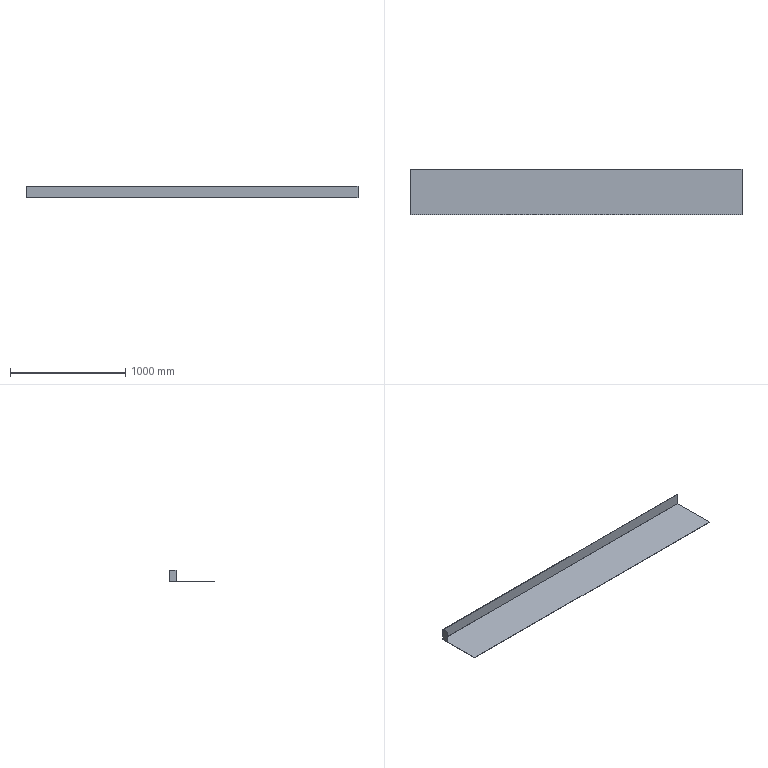Part | STEP file | PN_0036 third-floor site mounting plate 2_Default<As Machined> | 2 solids | 14 faces | box 2885 x 394 x 103 mm | volume 4292084 mm3 | plane 14
STEP:
#1=CARTESIAN_POINT('',(0.,0.,0.));
#2=DIRECTION('',(0.,0.,1.));
#3=DIRECTION('',(1.,0.,0.));
#4=AXIS2_PLACEMENT_3D('',#1,#2,#3);
#5=CARTESIAN_POINT('',(1442.5,-197.,0.));
#6=VERTEX_POINT('',#5);
#7=CARTESIAN_POINT('',(1442.5,197.,0.));
#8=VERTEX_POINT('',#7);
#9=CARTESIAN_POINT('',(1442.5,197.,0.));
#10=DIRECTION('',(0.,1.,0.));
#11=VECTOR('',#10,1.);
#12=LINE('',#9,#11);
#13=CARTESIAN_POINT('',(1442.5,197.,-3.));
#14=DIRECTION('',(1.,0.,0.));
#15=DIRECTION('',(0.,0.,-1.));
#16=AXIS2_PLACEMENT_3D('',#13,#14,#15);
#17=PLANE('',#16);
#18=CARTESIAN_POINT('',(-3.,0.));
#19=DIRECTION('',(0.,1.));
#20=VECTOR('',#19,1.);
#21=LINE('',#18,#20);
#22=(GEOMETRIC_REPRESENTATION_CONTEXT(2)PARAMETRIC_REPRESENTATION_CONTEXT()REPRESENTATION_CONTEXT('',''));
#23=DEFINITIONAL_REPRESENTATION('',(#21),#22);
#24=PCURVE('',#17,#23);
#25=CARTESIAN_POINT('',(0.,0.,0.));
#26=DIRECTION('',(0.,0.,1.));
#27=DIRECTION('',(1.,0.,0.));
#28=AXIS2_PLACEMENT_3D('',#25,#26,#27);
#29=PLANE('',#28);
#30=CARTESIAN_POINT('',(1442.5,197.));
#31=DIRECTION('',(0.,1.));
#32=VECTOR('',#31,1.);
#33=LINE('',#30,#32);
#34=(GEOMETRIC_REPRESENTATION_CONTEXT(2)PARAMETRIC_REPRESENTATION_CONTEXT()REPRESENTATION_CONTEXT('',''));
#35=DEFINITIONAL_REPRESENTATION('',(#33),#34);
#36=PCURVE('',#29,#35);
#37=SURFACE_CURVE('',#12,(#24,#36),.PCURVE_S1.);
#38=EDGE_CURVE('',#6,#8,#37,.T.);
#39=ORIENTED_EDGE('',*,*,#38,.F.);
#40=CARTESIAN_POINT('',(1442.5,-197.,-3.));
#41=VERTEX_POINT('',#40);
#42=CARTESIAN_POINT('',(1442.5,-197.,-3.));
#43=DIRECTION('',(0.,0.,1.));
#44=VECTOR('',#43,1.);
#45=LINE('',#42,#44);
#46=CARTESIAN_POINT('',(0.,-394.));
#47=DIRECTION('',(-1.,0.));
#48=VECTOR('',#47,1.);
#49=LINE('',#46,#48);
#50=(GEOMETRIC_REPRESENTATION_CONTEXT(2)PARAMETRIC_REPRESENTATION_CONTEXT()REPRESENTATION_CONTEXT('',''));
#51=DEFINITIONAL_REPRESENTATION('',(#49),#50);
#52=PCURVE('',#17,#51);
#53=CARTESIAN_POINT('',(-1442.5,-197.,-3.));
#54=DIRECTION('',(0.,-1.,0.));
#55=DIRECTION('',(0.,0.,-1.));
#56=AXIS2_PLACEMENT_3D('',#53,#54,#55);
#57=PLANE('',#56);
#58=CARTESIAN_POINT('',(0.,2885.));
#59=DIRECTION('',(-1.,0.));
#60=VECTOR('',#59,1.);
#61=LINE('',#58,#60);
#62=(GEOMETRIC_REPRESENTATION_CONTEXT(2)PARAMETRIC_REPRESENTATION_CONTEXT()REPRESENTATION_CONTEXT('',''));
#63=DEFINITIONAL_REPRESENTATION('',(#61),#62);
#64=PCURVE('',#57,#63);
#65=SURFACE_CURVE('',#45,(#52,#64),.PCURVE_S1.);
#66=EDGE_CURVE('',#41,#6,#65,.T.);
#67=ORIENTED_EDGE('',*,*,#66,.F.);
#68=CARTESIAN_POINT('',(1442.5,197.,-3.));
#69=VERTEX_POINT('',#68);
#70=CARTESIAN_POINT('',(1442.5,197.,-3.));
#71=DIRECTION('',(0.,1.,0.));
#72=VECTOR('',#71,1.);
#73=LINE('',#70,#72);
#74=CARTESIAN_POINT('',(0.,0.));
#75=DIRECTION('',(0.,1.));
#76=VECTOR('',#75,1.);
#77=LINE('',#74,#76);
#78=(GEOMETRIC_REPRESENTATION_CONTEXT(2)PARAMETRIC_REPRESENTATION_CONTEXT()REPRESENTATION_CONTEXT('',''));
#79=DEFINITIONAL_REPRESENTATION('',(#77),#78);
#80=PCURVE('',#17,#79);
#81=CARTESIAN_POINT('',(0.,0.,-3.));
#82=DIRECTION('',(0.,0.,1.));
#83=DIRECTION('',(1.,0.,0.));
#84=AXIS2_PLACEMENT_3D('',#81,#82,#83);
#85=PLANE('',#84);
#86=CARTESIAN_POINT('',(1442.5,197.));
#87=DIRECTION('',(0.,1.));
#88=VECTOR('',#87,1.);
#89=LINE('',#86,#88);
#90=(GEOMETRIC_REPRESENTATION_CONTEXT(2)PARAMETRIC_REPRESENTATION_CONTEXT()REPRESENTATION_CONTEXT('',''));
#91=DEFINITIONAL_REPRESENTATION('',(#89),#90);
#92=PCURVE('',#85,#91);
#93=SURFACE_CURVE('',#73,(#80,#92),.PCURVE_S1.);
#94=EDGE_CURVE('',#41,#69,#93,.T.);
#95=ORIENTED_EDGE('',*,*,#94,.T.);
#96=CARTESIAN_POINT('',(1442.5,197.,-3.));
#97=DIRECTION('',(0.,0.,1.));
#98=VECTOR('',#97,1.);
#99=LINE('',#96,#98);
#100=CARTESIAN_POINT('',(0.,0.));
#101=DIRECTION('',(-1.,0.));
#102=VECTOR('',#101,1.);
#103=LINE('',#100,#102);
#104=(GEOMETRIC_REPRESENTATION_CONTEXT(2)PARAMETRIC_REPRESENTATION_CONTEXT()REPRESENTATION_CONTEXT('',''));
#105=DEFINITIONAL_REPRESENTATION('',(#103),#104);
#106=PCURVE('',#17,#105);
#107=CARTESIAN_POINT('',(-1442.5,197.,-3.));
#108=DIRECTION('',(0.,1.,0.));
#109=DIRECTION('',(0.,0.,1.));
#110=AXIS2_PLACEMENT_3D('',#107,#108,#109);
#111=PLANE('',#110);
#112=CARTESIAN_POINT('',(0.,2885.));
#113=DIRECTION('',(1.,0.));
#114=VECTOR('',#113,1.);
#115=LINE('',#112,#114);
#116=(GEOMETRIC_REPRESENTATION_CONTEXT(2)PARAMETRIC_REPRESENTATION_CONTEXT()REPRESENTATION_CONTEXT('',''));
#117=DEFINITIONAL_REPRESENTATION('',(#115),#116);
#118=PCURVE('',#111,#117);
#119=SURFACE_CURVE('',#99,(#106,#118),.PCURVE_S1.);
#120=EDGE_CURVE('',#69,#8,#119,.T.);
#121=ORIENTED_EDGE('',*,*,#120,.T.);
#122=EDGE_LOOP('',(#39,#67,#95,#121));
#123=FACE_BOUND('',#122,.T.);
#124=ADVANCED_FACE('',(#123),#17,.T.);
#125=CARTESIAN_POINT('',(-1442.5,-197.,0.));
#126=VERTEX_POINT('',#125);
#127=CARTESIAN_POINT('',(-1442.5,-197.,0.));
#128=DIRECTION('',(1.,0.,0.));
#129=VECTOR('',#128,1.);
#130=LINE('',#127,#129);
#131=CARTESIAN_POINT('',(-3.,0.));
#132=DIRECTION('',(0.,1.));
#133=VECTOR('',#132,1.);
#134=LINE('',#131,#133);
#135=(GEOMETRIC_REPRESENTATION_CONTEXT(2)PARAMETRIC_REPRESENTATION_CONTEXT()REPRESENTATION_CONTEXT('',''));
#136=DEFINITIONAL_REPRESENTATION('',(#134),#135);
#137=PCURVE('',#57,#136);
#138=CARTESIAN_POINT('',(-1442.5,-197.));
#139=DIRECTION('',(1.,0.));
#140=VECTOR('',#139,1.);
#141=LINE('',#138,#140);
#142=(GEOMETRIC_REPRESENTATION_CONTEXT(2)PARAMETRIC_REPRESENTATION_CONTEXT()REPRESENTATION_CONTEXT('',''));
#143=DEFINITIONAL_REPRESENTATION('',(#141),#142);
#144=PCURVE('',#29,#143);
#145=SURFACE_CURVE('',#130,(#137,#144),.PCURVE_S1.);
#146=EDGE_CURVE('',#126,#6,#145,.T.);
#147=ORIENTED_EDGE('',*,*,#146,.F.);
#148=CARTESIAN_POINT('',(-1442.5,-197.,-3.));
#149=VERTEX_POINT('',#148);
#150=CARTESIAN_POINT('',(-1442.5,-197.,-3.));
#151=DIRECTION('',(0.,0.,1.));
#152=VECTOR('',#151,1.);
#153=LINE('',#150,#152);
#154=CARTESIAN_POINT('',(0.,0.));
#155=DIRECTION('',(-1.,0.));
#156=VECTOR('',#155,1.);
#157=LINE('',#154,#156);
#158=(GEOMETRIC_REPRESENTATION_CONTEXT(2)PARAMETRIC_REPRESENTATION_CONTEXT()REPRESENTATION_CONTEXT('',''));
#159=DEFINITIONAL_REPRESENTATION('',(#157),#158);
#160=PCURVE('',#57,#159);
#161=CARTESIAN_POINT('',(-1442.5,197.,-3.));
#162=DIRECTION('',(-1.,0.,0.));
#163=DIRECTION('',(0.,0.,1.));
#164=AXIS2_PLACEMENT_3D('',#161,#162,#163);
#165=PLANE('',#164);
#166=CARTESIAN_POINT('',(0.,-394.));
#167=DIRECTION('',(1.,0.));
#168=VECTOR('',#167,1.);
#169=LINE('',#166,#168);
#170=(GEOMETRIC_REPRESENTATION_CONTEXT(2)PARAMETRIC_REPRESENTATION_CONTEXT()REPRESENTATION_CONTEXT('',''));
#171=DEFINITIONAL_REPRESENTATION('',(#169),#170);
#172=PCURVE('',#165,#171);
#173=SURFACE_CURVE('',#153,(#160,#172),.PCURVE_S1.);
#174=EDGE_CURVE('',#149,#126,#173,.T.);
#175=ORIENTED_EDGE('',*,*,#174,.F.);
#176=CARTESIAN_POINT('',(-1442.5,-197.,-3.));
#177=DIRECTION('',(1.,0.,0.));
#178=VECTOR('',#177,1.);
#179=LINE('',#176,#178);
#180=CARTESIAN_POINT('',(0.,0.));
#181=DIRECTION('',(0.,1.));
#182=VECTOR('',#181,1.);
#183=LINE('',#180,#182);
#184=(GEOMETRIC_REPRESENTATION_CONTEXT(2)PARAMETRIC_REPRESENTATION_CONTEXT()REPRESENTATION_CONTEXT('',''));
#185=DEFINITIONAL_REPRESENTATION('',(#183),#184);
#186=PCURVE('',#57,#185);
#187=CARTESIAN_POINT('',(-1442.5,-197.));
#188=DIRECTION('',(1.,0.));
#189=VECTOR('',#188,1.);
#190=LINE('',#187,#189);
#191=(GEOMETRIC_REPRESENTATION_CONTEXT(2)PARAMETRIC_REPRESENTATION_CONTEXT()REPRESENTATION_CONTEXT('',''));
#192=DEFINITIONAL_REPRESENTATION('',(#190),#191);
#193=PCURVE('',#85,#192);
#194=SURFACE_CURVE('',#179,(#186,#193),.PCURVE_S1.);
#195=EDGE_CURVE('',#149,#41,#194,.T.);
#196=ORIENTED_EDGE('',*,*,#195,.T.);
#197=ORIENTED_EDGE('',*,*,#66,.T.);
#198=EDGE_LOOP('',(#147,#175,#196,#197));
#199=FACE_BOUND('',#198,.T.);
#200=ADVANCED_FACE('',(#199),#57,.T.);
#201=CARTESIAN_POINT('',(-1442.5,197.,0.));
#202=VERTEX_POINT('',#201);
#203=CARTESIAN_POINT('',(-1442.5,197.,0.));
#204=DIRECTION('',(0.,-1.,0.));
#205=VECTOR('',#204,1.);
#206=LINE('',#203,#205);
#207=CARTESIAN_POINT('',(3.,0.));
#208=DIRECTION('',(0.,-1.));
#209=VECTOR('',#208,1.);
#210=LINE('',#207,#209);
#211=(GEOMETRIC_REPRESENTATION_CONTEXT(2)PARAMETRIC_REPRESENTATION_CONTEXT()REPRESENTATION_CONTEXT('',''));
#212=DEFINITIONAL_REPRESENTATION('',(#210),#211);
#213=PCURVE('',#165,#212);
#214=CARTESIAN_POINT('',(-1442.5,197.));
#215=DIRECTION('',(0.,-1.));
#216=VECTOR('',#215,1.);
#217=LINE('',#214,#216);
#218=(GEOMETRIC_REPRESENTATION_CONTEXT(2)PARAMETRIC_REPRESENTATION_CONTEXT()REPRESENTATION_CONTEXT('',''));
#219=DEFINITIONAL_REPRESENTATION('',(#217),#218);
#220=PCURVE('',#29,#219);
#221=SURFACE_CURVE('',#206,(#213,#220),.PCURVE_S1.);
#222=EDGE_CURVE('',#202,#126,#221,.T.);
#223=ORIENTED_EDGE('',*,*,#222,.F.);
#224=CARTESIAN_POINT('',(-1442.5,197.,-3.));
#225=VERTEX_POINT('',#224);
#226=CARTESIAN_POINT('',(-1442.5,197.,-3.));
#227=DIRECTION('',(0.,0.,1.));
#228=VECTOR('',#227,1.);
#229=LINE('',#226,#228);
#230=CARTESIAN_POINT('',(0.,0.));
#231=DIRECTION('',(1.,0.));
#232=VECTOR('',#231,1.);
#233=LINE('',#230,#232);
#234=(GEOMETRIC_REPRESENTATION_CONTEXT(2)PARAMETRIC_REPRESENTATION_CONTEXT()REPRESENTATION_CONTEXT('',''));
#235=DEFINITIONAL_REPRESENTATION('',(#233),#234);
#236=PCURVE('',#165,#235);
#237=CARTESIAN_POINT('',(0.,0.));
#238=DIRECTION('',(1.,0.));
#239=VECTOR('',#238,1.);
#240=LINE('',#237,#239);
#241=(GEOMETRIC_REPRESENTATION_CONTEXT(2)PARAMETRIC_REPRESENTATION_CONTEXT()REPRESENTATION_CONTEXT('',''));
#242=DEFINITIONAL_REPRESENTATION('',(#240),#241);
#243=PCURVE('',#111,#242);
#244=SURFACE_CURVE('',#229,(#236,#243),.PCURVE_S1.);
#245=EDGE_CURVE('',#225,#202,#244,.T.);
#246=ORIENTED_EDGE('',*,*,#245,.F.);
#247=CARTESIAN_POINT('',(-1442.5,197.,-3.));
#248=DIRECTION('',(0.,-1.,0.));
#249=VECTOR('',#248,1.);
#250=LINE('',#247,#249);
#251=CARTESIAN_POINT('',(0.,0.));
#252=DIRECTION('',(0.,-1.));
#253=VECTOR('',#252,1.);
#254=LINE('',#251,#253);
#255=(GEOMETRIC_REPRESENTATION_CONTEXT(2)PARAMETRIC_REPRESENTATION_CONTEXT()REPRESENTATION_CONTEXT('',''));
#256=DEFINITIONAL_REPRESENTATION('',(#254),#255);
#257=PCURVE('',#165,#256);
#258=CARTESIAN_POINT('',(-1442.5,197.));
#259=DIRECTION('',(0.,-1.));
#260=VECTOR('',#259,1.);
#261=LINE('',#258,#260);
#262=(GEOMETRIC_REPRESENTATION_CONTEXT(2)PARAMETRIC_REPRESENTATION_CONTEXT()REPRESENTATION_CONTEXT('',''));
#263=DEFINITIONAL_REPRESENTATION('',(#261),#262);
#264=PCURVE('',#85,#263);
#265=SURFACE_CURVE('',#250,(#257,#264),.PCURVE_S1.);
#266=EDGE_CURVE('',#225,#149,#265,.T.);
#267=ORIENTED_EDGE('',*,*,#266,.T.);
#268=ORIENTED_EDGE('',*,*,#174,.T.);
#269=EDGE_LOOP('',(#223,#246,#267,#268));
#270=FACE_BOUND('',#269,.T.);
#271=ADVANCED_FACE('',(#270),#165,.T.);
#272=CARTESIAN_POINT('',(-1442.5,197.,0.));
#273=DIRECTION('',(-1.,0.,0.));
#274=VECTOR('',#273,1.);
#275=LINE('',#272,#274);
#276=CARTESIAN_POINT('',(3.,0.));
#277=DIRECTION('',(0.,-1.));
#278=VECTOR('',#277,1.);
#279=LINE('',#276,#278);
#280=(GEOMETRIC_REPRESENTATION_CONTEXT(2)PARAMETRIC_REPRESENTATION_CONTEXT()REPRESENTATION_CONTEXT('',''));
#281=DEFINITIONAL_REPRESENTATION('',(#279),#280);
#282=PCURVE('',#111,#281);
#283=CARTESIAN_POINT('',(-1442.5,197.));
#284=DIRECTION('',(-1.,0.));
#285=VECTOR('',#284,1.);
#286=LINE('',#283,#285);
#287=(GEOMETRIC_REPRESENTATION_CONTEXT(2)PARAMETRIC_REPRESENTATION_CONTEXT()REPRESENTATION_CONTEXT('',''));
#288=DEFINITIONAL_REPRESENTATION('',(#286),#287);
#289=PCURVE('',#29,#288);
#290=SURFACE_CURVE('',#275,(#282,#289),.PCURVE_S1.);
#291=EDGE_CURVE('',#8,#202,#290,.T.);
#292=ORIENTED_EDGE('',*,*,#291,.F.);
#293=ORIENTED_EDGE('',*,*,#120,.F.);
#294=CARTESIAN_POINT('',(-1442.5,197.,-3.));
#295=DIRECTION('',(-1.,0.,0.));
#296=VECTOR('',#295,1.);
#297=LINE('',#294,#296);
#298=CARTESIAN_POINT('',(0.,0.));
#299=DIRECTION('',(0.,-1.));
#300=VECTOR('',#299,1.);
#301=LINE('',#298,#300);
#302=(GEOMETRIC_REPRESENTATION_CONTEXT(2)PARAMETRIC_REPRESENTATION_CONTEXT()REPRESENTATION_CONTEXT('',''));
#303=DEFINITIONAL_REPRESENTATION('',(#301),#302);
#304=PCURVE('',#111,#303);
#305=CARTESIAN_POINT('',(-1442.5,197.));
#306=DIRECTION('',(-1.,0.));
#307=VECTOR('',#306,1.);
#308=LINE('',#305,#307);
#309=(GEOMETRIC_REPRESENTATION_CONTEXT(2)PARAMETRIC_REPRESENTATION_CONTEXT()REPRESENTATION_CONTEXT('',''));
#310=DEFINITIONAL_REPRESENTATION('',(#308),#309);
#311=PCURVE('',#85,#310);
#312=SURFACE_CURVE('',#297,(#304,#311),.PCURVE_S1.);
#313=EDGE_CURVE('',#69,#225,#312,.T.);
#314=ORIENTED_EDGE('',*,*,#313,.T.);
#315=ORIENTED_EDGE('',*,*,#245,.T.);
#316=EDGE_LOOP('',(#292,#293,#314,#315));
#317=FACE_BOUND('',#316,.T.);
#318=ADVANCED_FACE('',(#317),#111,.T.);
#319=ORIENTED_EDGE('',*,*,#94,.F.);
#320=ORIENTED_EDGE('',*,*,#195,.F.);
#321=ORIENTED_EDGE('',*,*,#266,.F.);
#322=ORIENTED_EDGE('',*,*,#313,.F.);
#323=EDGE_LOOP('',(#319,#320,#321,#322));
#324=FACE_BOUND('',#323,.T.);
#325=ADVANCED_FACE('',(#324),#85,.F.);
#326=ORIENTED_EDGE('',*,*,#38,.T.);
#327=ORIENTED_EDGE('',*,*,#291,.T.);
#328=ORIENTED_EDGE('',*,*,#222,.T.);
#329=ORIENTED_EDGE('',*,*,#146,.T.);
#330=EDGE_LOOP('',(#326,#327,#328,#329));
#331=FACE_BOUND('',#330,.T.);
#332=ADVANCED_FACE('',(#331),#29,.T.);
#333=CLOSED_SHELL('',(#124,#200,#271,#318,#325,#332));
#334=MANIFOLD_SOLID_BREP('',#333);
#335=CARTESIAN_POINT('',(-1442.5,197.,0.));
#336=VERTEX_POINT('',#335);
#337=CARTESIAN_POINT('',(-1442.5,138.955,0.));
#338=VERTEX_POINT('',#337);
#339=CARTESIAN_POINT('',(-1442.5,197.,0.));
#340=DIRECTION('',(0.,-1.,0.));
#341=VECTOR('',#340,1.);
#342=LINE('',#339,#341);
#343=CARTESIAN_POINT('',(-1442.5,197.,100.));
#344=DIRECTION('',(1.,0.,0.));
#345=DIRECTION('',(0.,0.,-1.));
#346=AXIS2_PLACEMENT_3D('',#343,#344,#345);
#347=PLANE('',#346);
#348=CARTESIAN_POINT('',(100.,0.));
#349=DIRECTION('',(0.,-1.));
#350=VECTOR('',#349,1.);
#351=LINE('',#348,#350);
#352=(GEOMETRIC_REPRESENTATION_CONTEXT(2)PARAMETRIC_REPRESENTATION_CONTEXT()REPRESENTATION_CONTEXT('',''));
#353=DEFINITIONAL_REPRESENTATION('',(#351),#352);
#354=PCURVE('',#347,#353);
#355=CARTESIAN_POINT('',(0.,0.,0.));
#356=DIRECTION('',(0.,0.,-1.));
#357=DIRECTION('',(-1.,0.,0.));
#358=AXIS2_PLACEMENT_3D('',#355,#356,#357);
#359=PLANE('',#358);
#360=CARTESIAN_POINT('',(1442.5,197.));
#361=DIRECTION('',(0.,-1.));
#362=VECTOR('',#361,1.);
#363=LINE('',#360,#362);
#364=(GEOMETRIC_REPRESENTATION_CONTEXT(2)PARAMETRIC_REPRESENTATION_CONTEXT()REPRESENTATION_CONTEXT('',''));
#365=DEFINITIONAL_REPRESENTATION('',(#363),#364);
#366=PCURVE('',#359,#365);
#367=SURFACE_CURVE('',#342,(#354,#366),.PCURVE_S1.);
#368=EDGE_CURVE('',#336,#338,#367,.T.);
#369=ORIENTED_EDGE('',*,*,#368,.T.);
#370=CARTESIAN_POINT('',(-1442.5,138.955,100.));
#371=VERTEX_POINT('',#370);
#372=CARTESIAN_POINT('',(-1442.5,138.955,100.));
#373=DIRECTION('',(0.,0.,-1.));
#374=VECTOR('',#373,1.);
#375=LINE('',#372,#374);
#376=CARTESIAN_POINT('',(0.,-58.045));
#377=DIRECTION('',(1.,0.));
#378=VECTOR('',#377,1.);
#379=LINE('',#376,#378);
#380=(GEOMETRIC_REPRESENTATION_CONTEXT(2)PARAMETRIC_REPRESENTATION_CONTEXT()REPRESENTATION_CONTEXT('',''));
#381=DEFINITIONAL_REPRESENTATION('',(#379),#380);
#382=PCURVE('',#347,#381);
#383=CARTESIAN_POINT('',(-1439.5,138.955,100.));
#384=DIRECTION('',(0.,-1.,0.));
#385=DIRECTION('',(0.,0.,-1.));
#386=AXIS2_PLACEMENT_3D('',#383,#384,#385);
#387=PLANE('',#386);
#388=CARTESIAN_POINT('',(0.,-3.));
#389=DIRECTION('',(1.,0.));
#390=VECTOR('',#389,1.);
#391=LINE('',#388,#390);
#392=(GEOMETRIC_REPRESENTATION_CONTEXT(2)PARAMETRIC_REPRESENTATION_CONTEXT()REPRESENTATION_CONTEXT('',''));
#393=DEFINITIONAL_REPRESENTATION('',(#391),#392);
#394=PCURVE('',#387,#393);
#395=SURFACE_CURVE('',#375,(#382,#394),.PCURVE_S1.);
#396=EDGE_CURVE('',#371,#338,#395,.T.);
#397=ORIENTED_EDGE('',*,*,#396,.F.);
#398=CARTESIAN_POINT('',(-1442.5,197.,100.));
#399=VERTEX_POINT('',#398);
#400=CARTESIAN_POINT('',(-1442.5,197.,100.));
#401=DIRECTION('',(0.,-1.,0.));
#402=VECTOR('',#401,1.);
#403=LINE('',#400,#402);
#404=CARTESIAN_POINT('',(0.,0.));
#405=DIRECTION('',(0.,-1.));
#406=VECTOR('',#405,1.);
#407=LINE('',#404,#406);
#408=(GEOMETRIC_REPRESENTATION_CONTEXT(2)PARAMETRIC_REPRESENTATION_CONTEXT()REPRESENTATION_CONTEXT('',''));
#409=DEFINITIONAL_REPRESENTATION('',(#407),#408);
#410=PCURVE('',#347,#409);
#411=CARTESIAN_POINT('',(0.,0.,100.));
#412=DIRECTION('',(0.,0.,-1.));
#413=DIRECTION('',(-1.,0.,0.));
#414=AXIS2_PLACEMENT_3D('',#411,#412,#413);
#415=PLANE('',#414);
#416=CARTESIAN_POINT('',(1442.5,197.));
#417=DIRECTION('',(0.,-1.));
#418=VECTOR('',#417,1.);
#419=LINE('',#416,#418);
#420=(GEOMETRIC_REPRESENTATION_CONTEXT(2)PARAMETRIC_REPRESENTATION_CONTEXT()REPRESENTATION_CONTEXT('',''));
#421=DEFINITIONAL_REPRESENTATION('',(#419),#420);
#422=PCURVE('',#415,#421);
#423=SURFACE_CURVE('',#403,(#410,#422),.PCURVE_S1.);
#424=EDGE_CURVE('',#399,#371,#423,.T.);
#425=ORIENTED_EDGE('',*,*,#424,.F.);
#426=CARTESIAN_POINT('',(-1442.5,197.,100.));
#427=DIRECTION('',(0.,0.,-1.));
#428=VECTOR('',#427,1.);
#429=LINE('',#426,#428);
#430=CARTESIAN_POINT('',(0.,0.));
#431=DIRECTION('',(1.,0.));
#432=VECTOR('',#431,1.);
#433=LINE('',#430,#432);
#434=(GEOMETRIC_REPRESENTATION_CONTEXT(2)PARAMETRIC_REPRESENTATION_CONTEXT()REPRESENTATION_CONTEXT('',''));
#435=DEFINITIONAL_REPRESENTATION('',(#433),#434);
#436=PCURVE('',#347,#435);
#437=CARTESIAN_POINT('',(-1442.5,197.,100.));
#438=DIRECTION('',(0.,-1.,0.));
#439=DIRECTION('',(0.,0.,-1.));
#440=AXIS2_PLACEMENT_3D('',#437,#438,#439);
#441=PLANE('',#440);
#442=CARTESIAN_POINT('',(0.,0.));
#443=DIRECTION('',(1.,0.));
#444=VECTOR('',#443,1.);
#445=LINE('',#442,#444);
#446=(GEOMETRIC_REPRESENTATION_CONTEXT(2)PARAMETRIC_REPRESENTATION_CONTEXT()REPRESENTATION_CONTEXT('',''));
#447=DEFINITIONAL_REPRESENTATION('',(#445),#446);
#448=PCURVE('',#441,#447);
#449=SURFACE_CURVE('',#429,(#436,#448),.PCURVE_S1.);
#450=EDGE_CURVE('',#399,#336,#449,.T.);
#451=ORIENTED_EDGE('',*,*,#450,.T.);
#452=EDGE_LOOP('',(#369,#397,#425,#451));
#453=FACE_BOUND('',#452,.T.);
#454=ADVANCED_FACE('',(#453),#347,.F.);
#455=CARTESIAN_POINT('',(-1439.5,138.955,0.));
#456=VERTEX_POINT('',#455);
#457=CARTESIAN_POINT('',(-1439.5,138.955,0.));
#458=DIRECTION('',(-1.,0.,0.));
#459=VECTOR('',#458,1.);
#460=LINE('',#457,#459);
#461=CARTESIAN_POINT('',(100.,0.));
#462=DIRECTION('',(0.,-1.));
#463=VECTOR('',#462,1.);
#464=LINE('',#461,#463);
#465=(GEOMETRIC_REPRESENTATION_CONTEXT(2)PARAMETRIC_REPRESENTATION_CONTEXT()REPRESENTATION_CONTEXT('',''));
#466=DEFINITIONAL_REPRESENTATION('',(#464),#465);
#467=PCURVE('',#387,#466);
#468=CARTESIAN_POINT('',(1439.5,138.955));
#469=DIRECTION('',(1.,0.));
#470=VECTOR('',#469,1.);
#471=LINE('',#468,#470);
#472=(GEOMETRIC_REPRESENTATION_CONTEXT(2)PARAMETRIC_REPRESENTATION_CONTEXT()REPRESENTATION_CONTEXT('',''));
#473=DEFINITIONAL_REPRESENTATION('',(#471),#472);
#474=PCURVE('',#359,#473);
#475=SURFACE_CURVE('',#460,(#467,#474),.PCURVE_S1.);
#476=EDGE_CURVE('',#456,#338,#475,.T.);
#477=ORIENTED_EDGE('',*,*,#476,.F.);
#478=CARTESIAN_POINT('',(-1439.5,138.955,100.));
#479=VERTEX_POINT('',#478);
#480=CARTESIAN_POINT('',(-1439.5,138.955,100.));
#481=DIRECTION('',(0.,0.,-1.));
#482=VECTOR('',#481,1.);
#483=LINE('',#480,#482);
#484=CARTESIAN_POINT('',(0.,0.));
#485=DIRECTION('',(1.,0.));
#486=VECTOR('',#485,1.);
#487=LINE('',#484,#486);
#488=(GEOMETRIC_REPRESENTATION_CONTEXT(2)PARAMETRIC_REPRESENTATION_CONTEXT()REPRESENTATION_CONTEXT('',''));
#489=DEFINITIONAL_REPRESENTATION('',(#487),#488);
#490=PCURVE('',#387,#489);
#491=CARTESIAN_POINT('',(-1439.5,197.,100.));
#492=DIRECTION('',(1.,0.,0.));
#493=DIRECTION('',(0.,0.,-1.));
#494=AXIS2_PLACEMENT_3D('',#491,#492,#493);
#495=PLANE('',#494);
#496=CARTESIAN_POINT('',(0.,-58.045));
#497=DIRECTION('',(1.,0.));
#498=VECTOR('',#497,1.);
#499=LINE('',#496,#498);
#500=(GEOMETRIC_REPRESENTATION_CONTEXT(2)PARAMETRIC_REPRESENTATION_CONTEXT()REPRESENTATION_CONTEXT('',''));
#501=DEFINITIONAL_REPRESENTATION('',(#499),#500);
#502=PCURVE('',#495,#501);
#503=SURFACE_CURVE('',#483,(#490,#502),.PCURVE_S1.);
#504=EDGE_CURVE('',#479,#456,#503,.T.);
#505=ORIENTED_EDGE('',*,*,#504,.F.);
#506=CARTESIAN_POINT('',(-1439.5,138.955,100.));
#507=DIRECTION('',(-1.,0.,0.));
#508=VECTOR('',#507,1.);
#509=LINE('',#506,#508);
#510=CARTESIAN_POINT('',(0.,0.));
#511=DIRECTION('',(0.,-1.));
#512=VECTOR('',#511,1.);
#513=LINE('',#510,#512);
#514=(GEOMETRIC_REPRESENTATION_CONTEXT(2)PARAMETRIC_REPRESENTATION_CONTEXT()REPRESENTATION_CONTEXT('',''));
#515=DEFINITIONAL_REPRESENTATION('',(#513),#514);
#516=PCURVE('',#387,#515);
#517=CARTESIAN_POINT('',(1439.5,138.955));
#518=DIRECTION('',(1.,0.));
#519=VECTOR('',#518,1.);
#520=LINE('',#517,#519);
#521=(GEOMETRIC_REPRESENTATION_CONTEXT(2)PARAMETRIC_REPRESENTATION_CONTEXT()REPRESENTATION_CONTEXT('',''));
#522=DEFINITIONAL_REPRESENTATION('',(#520),#521);
#523=PCURVE('',#415,#522);
#524=SURFACE_CURVE('',#509,(#516,#523),.PCURVE_S1.);
#525=EDGE_CURVE('',#479,#371,#524,.T.);
#526=ORIENTED_EDGE('',*,*,#525,.T.);
#527=ORIENTED_EDGE('',*,*,#396,.T.);
#528=EDGE_LOOP('',(#477,#505,#526,#527));
#529=FACE_BOUND('',#528,.T.);
#530=ADVANCED_FACE('',(#529),#387,.T.);
#531=CARTESIAN_POINT('',(-1439.5,194.,0.));
#532=VERTEX_POINT('',#531);
#533=CARTESIAN_POINT('',(-1439.5,197.,0.));
#534=DIRECTION('',(0.,-1.,0.));
#535=VECTOR('',#534,1.);
#536=LINE('',#533,#535);
#537=CARTESIAN_POINT('',(100.,0.));
#538=DIRECTION('',(0.,-1.));
#539=VECTOR('',#538,1.);
#540=LINE('',#537,#539);
#541=(GEOMETRIC_REPRESENTATION_CONTEXT(2)PARAMETRIC_REPRESENTATION_CONTEXT()REPRESENTATION_CONTEXT('',''));
#542=DEFINITIONAL_REPRESENTATION('',(#540),#541);
#543=PCURVE('',#495,#542);
#544=CARTESIAN_POINT('',(1439.5,197.));
#545=DIRECTION('',(0.,-1.));
#546=VECTOR('',#545,1.);
#547=LINE('',#544,#546);
#548=(GEOMETRIC_REPRESENTATION_CONTEXT(2)PARAMETRIC_REPRESENTATION_CONTEXT()REPRESENTATION_CONTEXT('',''));
#549=DEFINITIONAL_REPRESENTATION('',(#547),#548);
#550=PCURVE('',#359,#549);
#551=SURFACE_CURVE('',#536,(#543,#550),.PCURVE_S1.);
#552=EDGE_CURVE('',#532,#456,#551,.T.);
#553=ORIENTED_EDGE('',*,*,#552,.F.);
#554=CARTESIAN_POINT('',(-1439.5,194.,100.));
#555=VERTEX_POINT('',#554);
#556=CARTESIAN_POINT('',(-1439.5,194.,100.));
#557=DIRECTION('',(0.,0.,-1.));
#558=VECTOR('',#557,1.);
#559=LINE('',#556,#558);
#560=CARTESIAN_POINT('',(0.,-3.));
#561=DIRECTION('',(1.,0.));
#562=VECTOR('',#561,1.);
#563=LINE('',#560,#562);
#564=(GEOMETRIC_REPRESENTATION_CONTEXT(2)PARAMETRIC_REPRESENTATION_CONTEXT()REPRESENTATION_CONTEXT('',''));
#565=DEFINITIONAL_REPRESENTATION('',(#563),#564);
#566=PCURVE('',#495,#565);
#567=CARTESIAN_POINT('',(-1442.5,194.,100.));
#568=DIRECTION('',(0.,-1.,0.));
#569=DIRECTION('',(0.,0.,-1.));
#570=AXIS2_PLACEMENT_3D('',#567,#568,#569);
#571=PLANE('',#570);
#572=CARTESIAN_POINT('',(0.,3.));
#573=DIRECTION('',(1.,0.));
#574=VECTOR('',#573,1.);
#575=LINE('',#572,#574);
#576=(GEOMETRIC_REPRESENTATION_CONTEXT(2)PARAMETRIC_REPRESENTATION_CONTEXT()REPRESENTATION_CONTEXT('',''));
#577=DEFINITIONAL_REPRESENTATION('',(#575),#576);
#578=PCURVE('',#571,#577);
#579=SURFACE_CURVE('',#559,(#566,#578),.PCURVE_S1.);
#580=EDGE_CURVE('',#555,#532,#579,.T.);
#581=ORIENTED_EDGE('',*,*,#580,.F.);
#582=CARTESIAN_POINT('',(-1439.5,197.,100.));
#583=DIRECTION('',(0.,-1.,0.));
#584=VECTOR('',#583,1.);
#585=LINE('',#582,#584);
#586=CARTESIAN_POINT('',(0.,0.));
#587=DIRECTION('',(0.,-1.));
#588=VECTOR('',#587,1.);
#589=LINE('',#586,#588);
#590=(GEOMETRIC_REPRESENTATION_CONTEXT(2)PARAMETRIC_REPRESENTATION_CONTEXT()REPRESENTATION_CONTEXT('',''));
#591=DEFINITIONAL_REPRESENTATION('',(#589),#590);
#592=PCURVE('',#495,#591);
#593=CARTESIAN_POINT('',(1439.5,197.));
#594=DIRECTION('',(0.,-1.));
#595=VECTOR('',#594,1.);
#596=LINE('',#593,#595);
#597=(GEOMETRIC_REPRESENTATION_CONTEXT(2)PARAMETRIC_REPRESENTATION_CONTEXT()REPRESENTATION_CONTEXT('',''));
#598=DEFINITIONAL_REPRESENTATION('',(#596),#597);
#599=PCURVE('',#415,#598);
#600=SURFACE_CURVE('',#585,(#592,#599),.PCURVE_S1.);
#601=EDGE_CURVE('',#555,#479,#600,.T.);
#602=ORIENTED_EDGE('',*,*,#601,.T.);
#603=ORIENTED_EDGE('',*,*,#504,.T.);
#604=EDGE_LOOP('',(#553,#581,#602,#603));
#605=FACE_BOUND('',#604,.T.);
#606=ADVANCED_FACE('',(#605),#495,.T.);
#607=CARTESIAN_POINT('',(1442.5,194.,0.));
#608=VERTEX_POINT('',#607);
#609=CARTESIAN_POINT('',(-1442.5,194.,0.));
#610=DIRECTION('',(-1.,0.,0.));
#611=VECTOR('',#610,1.);
#612=LINE('',#609,#611);
#613=CARTESIAN_POINT('',(100.,0.));
#614=DIRECTION('',(0.,-1.));
#615=VECTOR('',#614,1.);
#616=LINE('',#613,#615);
#617=(GEOMETRIC_REPRESENTATION_CONTEXT(2)PARAMETRIC_REPRESENTATION_CONTEXT()REPRESENTATION_CONTEXT('',''));
#618=DEFINITIONAL_REPRESENTATION('',(#616),#617);
#619=PCURVE('',#571,#618);
#620=CARTESIAN_POINT('',(1442.5,194.));
#621=DIRECTION('',(1.,0.));
#622=VECTOR('',#621,1.);
#623=LINE('',#620,#622);
#624=(GEOMETRIC_REPRESENTATION_CONTEXT(2)PARAMETRIC_REPRESENTATION_CONTEXT()REPRESENTATION_CONTEXT('',''));
#625=DEFINITIONAL_REPRESENTATION('',(#623),#624);
#626=PCURVE('',#359,#625);
#627=SURFACE_CURVE('',#612,(#619,#626),.PCURVE_S1.);
#628=EDGE_CURVE('',#608,#532,#627,.T.);
#629=ORIENTED_EDGE('',*,*,#628,.F.);
#630=CARTESIAN_POINT('',(1442.5,194.,100.));
#631=VERTEX_POINT('',#630);
#632=CARTESIAN_POINT('',(1442.5,194.,100.));
#633=DIRECTION('',(0.,0.,-1.));
#634=VECTOR('',#633,1.);
#635=LINE('',#632,#634);
#636=CARTESIAN_POINT('',(0.,2885.));
#637=DIRECTION('',(1.,0.));
#638=VECTOR('',#637,1.);
#639=LINE('',#636,#638);
#640=(GEOMETRIC_REPRESENTATION_CONTEXT(2)PARAMETRIC_REPRESENTATION_CONTEXT()REPRESENTATION_CONTEXT('',''));
#641=DEFINITIONAL_REPRESENTATION('',(#639),#640);
#642=PCURVE('',#571,#641);
#643=CARTESIAN_POINT('',(1442.5,197.,100.));
#644=DIRECTION('',(1.,0.,0.));
#645=DIRECTION('',(0.,0.,-1.));
#646=AXIS2_PLACEMENT_3D('',#643,#644,#645);
#647=PLANE('',#646);
#648=CARTESIAN_POINT('',(0.,-3.));
#649=DIRECTION('',(1.,0.));
#650=VECTOR('',#649,1.);
#651=LINE('',#648,#650);
#652=(GEOMETRIC_REPRESENTATION_CONTEXT(2)PARAMETRIC_REPRESENTATION_CONTEXT()REPRESENTATION_CONTEXT('',''));
#653=DEFINITIONAL_REPRESENTATION('',(#651),#652);
#654=PCURVE('',#647,#653);
#655=SURFACE_CURVE('',#635,(#642,#654),.PCURVE_S1.);
#656=EDGE_CURVE('',#631,#608,#655,.T.);
#657=ORIENTED_EDGE('',*,*,#656,.F.);
#658=CARTESIAN_POINT('',(-1442.5,194.,100.));
#659=DIRECTION('',(-1.,0.,0.));
#660=VECTOR('',#659,1.);
#661=LINE('',#658,#660);
#662=CARTESIAN_POINT('',(0.,0.));
#663=DIRECTION('',(0.,-1.));
#664=VECTOR('',#663,1.);
#665=LINE('',#662,#664);
#666=(GEOMETRIC_REPRESENTATION_CONTEXT(2)PARAMETRIC_REPRESENTATION_CONTEXT()REPRESENTATION_CONTEXT('',''));
#667=DEFINITIONAL_REPRESENTATION('',(#665),#666);
#668=PCURVE('',#571,#667);
#669=CARTESIAN_POINT('',(1442.5,194.));
#670=DIRECTION('',(1.,0.));
#671=VECTOR('',#670,1.);
#672=LINE('',#669,#671);
#673=(GEOMETRIC_REPRESENTATION_CONTEXT(2)PARAMETRIC_REPRESENTATION_CONTEXT()REPRESENTATION_CONTEXT('',''));
#674=DEFINITIONAL_REPRESENTATION('',(#672),#673);
#675=PCURVE('',#415,#674);
#676=SURFACE_CURVE('',#661,(#668,#675),.PCURVE_S1.);
#677=EDGE_CURVE('',#631,#555,#676,.T.);
#678=ORIENTED_EDGE('',*,*,#677,.T.);
#679=ORIENTED_EDGE('',*,*,#580,.T.);
#680=EDGE_LOOP('',(#629,#657,#678,#679));
#681=FACE_BOUND('',#680,.T.);
#682=ADVANCED_FACE('',(#681),#571,.T.);
#683=CARTESIAN_POINT('',(1442.5,197.,0.));
#684=VERTEX_POINT('',#683);
#685=CARTESIAN_POINT('',(1442.5,197.,0.));
#686=DIRECTION('',(0.,-1.,0.));
#687=VECTOR('',#686,1.);
#688=LINE('',#685,#687);
#689=CARTESIAN_POINT('',(100.,0.));
#690=DIRECTION('',(0.,-1.));
#691=VECTOR('',#690,1.);
#692=LINE('',#689,#691);
#693=(GEOMETRIC_REPRESENTATION_CONTEXT(2)PARAMETRIC_REPRESENTATION_CONTEXT()REPRESENTATION_CONTEXT('',''));
#694=DEFINITIONAL_REPRESENTATION('',(#692),#693);
#695=PCURVE('',#647,#694);
#696=CARTESIAN_POINT('',(-1442.5,197.));
#697=DIRECTION('',(0.,-1.));
#698=VECTOR('',#697,1.);
#699=LINE('',#696,#698);
#700=(GEOMETRIC_REPRESENTATION_CONTEXT(2)PARAMETRIC_REPRESENTATION_CONTEXT()REPRESENTATION_CONTEXT('',''));
#701=DEFINITIONAL_REPRESENTATION('',(#699),#700);
#702=PCURVE('',#359,#701);
#703=SURFACE_CURVE('',#688,(#695,#702),.PCURVE_S1.);
#704=EDGE_CURVE('',#684,#608,#703,.T.);
#705=ORIENTED_EDGE('',*,*,#704,.F.);
#706=CARTESIAN_POINT('',(1442.5,197.,100.));
#707=VERTEX_POINT('',#706);
#708=CARTESIAN_POINT('',(1442.5,197.,100.));
#709=DIRECTION('',(0.,0.,-1.));
#710=VECTOR('',#709,1.);
#711=LINE('',#708,#710);
#712=CARTESIAN_POINT('',(0.,0.));
#713=DIRECTION('',(1.,0.));
#714=VECTOR('',#713,1.);
#715=LINE('',#712,#714);
#716=(GEOMETRIC_REPRESENTATION_CONTEXT(2)PARAMETRIC_REPRESENTATION_CONTEXT()REPRESENTATION_CONTEXT('',''));
#717=DEFINITIONAL_REPRESENTATION('',(#715),#716);
#718=PCURVE('',#647,#717);
#719=CARTESIAN_POINT('',(0.,2885.));
#720=DIRECTION('',(1.,0.));
#721=VECTOR('',#720,1.);
#722=LINE('',#719,#721);
#723=(GEOMETRIC_REPRESENTATION_CONTEXT(2)PARAMETRIC_REPRESENTATION_CONTEXT()REPRESENTATION_CONTEXT('',''));
#724=DEFINITIONAL_REPRESENTATION('',(#722),#723);
#725=PCURVE('',#441,#724);
#726=SURFACE_CURVE('',#711,(#718,#725),.PCURVE_S1.);
#727=EDGE_CURVE('',#707,#684,#726,.T.);
#728=ORIENTED_EDGE('',*,*,#727,.F.);
#729=CARTESIAN_POINT('',(1442.5,197.,100.));
#730=DIRECTION('',(0.,-1.,0.));
#731=VECTOR('',#730,1.);
#732=LINE('',#729,#731);
#733=CARTESIAN_POINT('',(0.,0.));
#734=DIRECTION('',(0.,-1.));
#735=VECTOR('',#734,1.);
#736=LINE('',#733,#735);
#737=(GEOMETRIC_REPRESENTATION_CONTEXT(2)PARAMETRIC_REPRESENTATION_CONTEXT()REPRESENTATION_CONTEXT('',''));
#738=DEFINITIONAL_REPRESENTATION('',(#736),#737);
#739=PCURVE('',#647,#738);
#740=CARTESIAN_POINT('',(-1442.5,197.));
#741=DIRECTION('',(0.,-1.));
#742=VECTOR('',#741,1.);
#743=LINE('',#740,#742);
#744=(GEOMETRIC_REPRESENTATION_CONTEXT(2)PARAMETRIC_REPRESENTATION_CONTEXT()REPRESENTATION_CONTEXT('',''));
#745=DEFINITIONAL_REPRESENTATION('',(#743),#744);
#746=PCURVE('',#415,#745);
#747=SURFACE_CURVE('',#732,(#739,#746),.PCURVE_S1.);
#748=EDGE_CURVE('',#707,#631,#747,.T.);
#749=ORIENTED_EDGE('',*,*,#748,.T.);
#750=ORIENTED_EDGE('',*,*,#656,.T.);
#751=EDGE_LOOP('',(#705,#728,#749,#750));
#752=FACE_BOUND('',#751,.T.);
#753=ADVANCED_FACE('',(#752),#647,.T.);
#754=CARTESIAN_POINT('',(-1442.5,197.,0.));
#755=DIRECTION('',(-1.,0.,0.));
#756=VECTOR('',#755,1.);
#757=LINE('',#754,#756);
#758=CARTESIAN_POINT('',(100.,0.));
#759=DIRECTION('',(0.,-1.));
#760=VECTOR('',#759,1.);
#761=LINE('',#758,#760);
#762=(GEOMETRIC_REPRESENTATION_CONTEXT(2)PARAMETRIC_REPRESENTATION_CONTEXT()REPRESENTATION_CONTEXT('',''));
#763=DEFINITIONAL_REPRESENTATION('',(#761),#762);
#764=PCURVE('',#441,#763);
#765=CARTESIAN_POINT('',(1442.5,197.));
#766=DIRECTION('',(1.,0.));
#767=VECTOR('',#766,1.);
#768=LINE('',#765,#767);
#769=(GEOMETRIC_REPRESENTATION_CONTEXT(2)PARAMETRIC_REPRESENTATION_CONTEXT()REPRESENTATION_CONTEXT('',''));
#770=DEFINITIONAL_REPRESENTATION('',(#768),#769);
#771=PCURVE('',#359,#770);
#772=SURFACE_CURVE('',#757,(#764,#771),.PCURVE_S1.);
#773=EDGE_CURVE('',#684,#336,#772,.T.);
#774=ORIENTED_EDGE('',*,*,#773,.T.);
#775=ORIENTED_EDGE('',*,*,#450,.F.);
#776=CARTESIAN_POINT('',(-1442.5,197.,100.));
#777=DIRECTION('',(-1.,0.,0.));
#778=VECTOR('',#777,1.);
#779=LINE('',#776,#778);
#780=CARTESIAN_POINT('',(0.,0.));
#781=DIRECTION('',(0.,-1.));
#782=VECTOR('',#781,1.);
#783=LINE('',#780,#782);
#784=(GEOMETRIC_REPRESENTATION_CONTEXT(2)PARAMETRIC_REPRESENTATION_CONTEXT()REPRESENTATION_CONTEXT('',''));
#785=DEFINITIONAL_REPRESENTATION('',(#783),#784);
#786=PCURVE('',#441,#785);
#787=CARTESIAN_POINT('',(1442.5,197.));
#788=DIRECTION('',(1.,0.));
#789=VECTOR('',#788,1.);
#790=LINE('',#787,#789);
#791=(GEOMETRIC_REPRESENTATION_CONTEXT(2)PARAMETRIC_REPRESENTATION_CONTEXT()REPRESENTATION_CONTEXT('',''));
#792=DEFINITIONAL_REPRESENTATION('',(#790),#791);
#793=PCURVE('',#415,#792);
#794=SURFACE_CURVE('',#779,(#786,#793),.PCURVE_S1.);
#795=EDGE_CURVE('',#707,#399,#794,.T.);
#796=ORIENTED_EDGE('',*,*,#795,.F.);
#797=ORIENTED_EDGE('',*,*,#727,.T.);
#798=EDGE_LOOP('',(#774,#775,#796,#797));
#799=FACE_BOUND('',#798,.T.);
#800=ADVANCED_FACE('',(#799),#441,.F.);
#801=ORIENTED_EDGE('',*,*,#424,.T.);
#802=ORIENTED_EDGE('',*,*,#525,.F.);
#803=ORIENTED_EDGE('',*,*,#601,.F.);
#804=ORIENTED_EDGE('',*,*,#677,.F.);
#805=ORIENTED_EDGE('',*,*,#748,.F.);
#806=ORIENTED_EDGE('',*,*,#795,.T.);
#807=EDGE_LOOP('',(#801,#802,#803,#804,#805,#806));
#808=FACE_BOUND('',#807,.T.);
#809=ADVANCED_FACE('',(#808),#415,.F.);
#810=ORIENTED_EDGE('',*,*,#368,.F.);
#811=ORIENTED_EDGE('',*,*,#773,.F.);
#812=ORIENTED_EDGE('',*,*,#704,.T.);
#813=ORIENTED_EDGE('',*,*,#628,.T.);
#814=ORIENTED_EDGE('',*,*,#552,.T.);
#815=ORIENTED_EDGE('',*,*,#476,.T.);
#816=EDGE_LOOP('',(#810,#811,#812,#813,#814,#815));
#817=FACE_BOUND('',#816,.T.);
#818=ADVANCED_FACE('',(#817),#359,.T.);
#819=CLOSED_SHELL('',(#454,#530,#606,#682,#753,#800,#809,#818));
#820=MANIFOLD_SOLID_BREP('',#819);
#821=(LENGTH_UNIT()NAMED_UNIT(*)SI_UNIT(.MILLI.,.METRE.));
#822=UNCERTAINTY_MEASURE_WITH_UNIT(LENGTH_MEASURE(0.0000001),#821,'','');
#823=(NAMED_UNIT(*)PLANE_ANGLE_UNIT()SI_UNIT($,.RADIAN.));
#824=(NAMED_UNIT(*)SI_UNIT($,.STERADIAN.)SOLID_ANGLE_UNIT());
#825=(GEOMETRIC_REPRESENTATION_CONTEXT(3)GLOBAL_UNCERTAINTY_ASSIGNED_CONTEXT((#822))GLOBAL_UNIT_ASSIGNED_CONTEXT((#821,#823,#824))REPRESENTATION_CONTEXT('',''));
#826=SHAPE_REPRESENTATION('',(#4,#334,#820),#825);